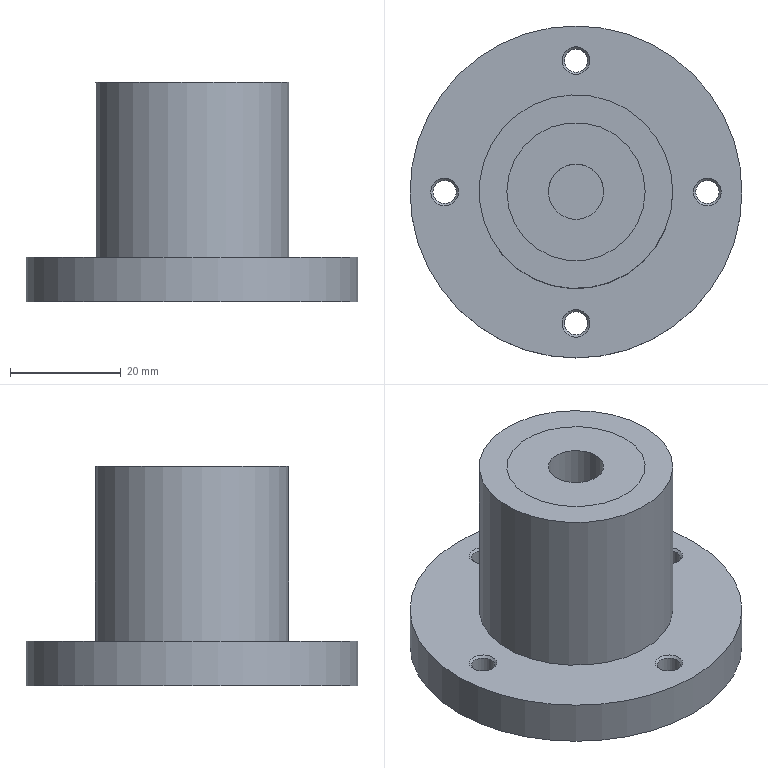Part | NX | features DATUM_CSYS 7, SKETCH 6, EXTRUDE 5, SIMPLE HOLE 4, SYMBOLIC_THREAD 4, HOLE PACKAGE 1 | 2 solids | 25 faces | box 60 x 60 x 39.6 mm | volume 47983 mm3 | cylinder 10 | cone 8 | plane 7 | commonest cylinder face diameters 4.2 x4 25 x2 10 x1 22 x1 35 x1 60 x1
STEP:
#1=CARTESIAN_POINT('',(30.,0.,8.));
#2=VERTEX_POINT('',#1);
#3=CARTESIAN_POINT('',(0.,0.,8.));
#4=DIRECTION('',(0.,0.,1.));
#5=DIRECTION('',(1.,0.,0.));
#6=AXIS2_PLACEMENT_3D('',#3,#4,#5);
#7=CIRCLE('',#6,30.);
#8=EDGE_CURVE('',#2,#2,#7,.T.);
#9=ORIENTED_EDGE('',*,*,#8,.F.);
#10=EDGE_LOOP('',(#9));
#11=FACE_BOUND('',#10,.T.);
#12=CARTESIAN_POINT('',(30.,0.,0.));
#13=VERTEX_POINT('',#12);
#14=CARTESIAN_POINT('',(0.,0.,0.));
#15=DIRECTION('',(0.,0.,1.));
#16=DIRECTION('',(1.,0.,0.));
#17=AXIS2_PLACEMENT_3D('',#14,#15,#16);
#18=CIRCLE('',#17,30.);
#19=EDGE_CURVE('',#13,#13,#18,.T.);
#20=ORIENTED_EDGE('',*,*,#19,.T.);
#21=EDGE_LOOP('',(#20));
#22=FACE_BOUND('',#21,.T.);
#23=CARTESIAN_POINT('',(0.,0.,8.));
#24=DIRECTION('',(0.,0.,-1.));
#25=DIRECTION('',(-1.,0.,0.));
#26=AXIS2_PLACEMENT_3D('',#23,#24,#25);
#27=CYLINDRICAL_SURFACE('',#26,30.);
#28=ADVANCED_FACE('',(#11,#22),#27,.T.);
#29=CARTESIAN_POINT('',(26.25,-0.00006047,8.));
#30=VERTEX_POINT('',#29);
#31=CARTESIAN_POINT('',(23.75,-0.00006047,8.));
#32=DIRECTION('',(0.,0.,1.));
#33=DIRECTION('',(1.,0.,0.));
#34=AXIS2_PLACEMENT_3D('',#31,#32,#33);
#35=CIRCLE('',#34,2.5);
#36=EDGE_CURVE('',#30,#30,#35,.F.);
#37=ORIENTED_EDGE('',*,*,#36,.T.);
#38=EDGE_LOOP('',(#37));
#39=FACE_BOUND('',#38,.T.);
#40=CARTESIAN_POINT('',(2.5,23.75,8.));
#41=VERTEX_POINT('',#40);
#42=CARTESIAN_POINT('',(0.00006047,23.75,8.));
#43=DIRECTION('',(0.,0.,1.));
#44=DIRECTION('',(1.,0.,0.));
#45=AXIS2_PLACEMENT_3D('',#42,#43,#44);
#46=CIRCLE('',#45,2.5);
#47=EDGE_CURVE('',#41,#41,#46,.F.);
#48=ORIENTED_EDGE('',*,*,#47,.T.);
#49=EDGE_LOOP('',(#48));
#50=FACE_BOUND('',#49,.T.);
#51=CARTESIAN_POINT('',(2.5,-23.75,8.));
#52=VERTEX_POINT('',#51);
#53=CARTESIAN_POINT('',(-0.00006047,-23.75,8.));
#54=DIRECTION('',(0.,0.,1.));
#55=DIRECTION('',(1.,0.,0.));
#56=AXIS2_PLACEMENT_3D('',#53,#54,#55);
#57=CIRCLE('',#56,2.5);
#58=EDGE_CURVE('',#52,#52,#57,.F.);
#59=ORIENTED_EDGE('',*,*,#58,.T.);
#60=EDGE_LOOP('',(#59));
#61=FACE_BOUND('',#60,.T.);
#62=CARTESIAN_POINT('',(-21.25,0.00006047,8.));
#63=VERTEX_POINT('',#62);
#64=CARTESIAN_POINT('',(-23.75,0.00006047,8.));
#65=DIRECTION('',(0.,0.,1.));
#66=DIRECTION('',(1.,0.,0.));
#67=AXIS2_PLACEMENT_3D('',#64,#65,#66);
#68=CIRCLE('',#67,2.5);
#69=EDGE_CURVE('',#63,#63,#68,.F.);
#70=ORIENTED_EDGE('',*,*,#69,.T.);
#71=EDGE_LOOP('',(#70));
#72=FACE_BOUND('',#71,.T.);
#73=CARTESIAN_POINT('',(17.5,0.,8.));
#74=VERTEX_POINT('',#73);
#75=CARTESIAN_POINT('',(0.,0.,8.));
#76=DIRECTION('',(0.,0.,1.));
#77=DIRECTION('',(1.,0.,0.));
#78=AXIS2_PLACEMENT_3D('',#75,#76,#77);
#79=CIRCLE('',#78,17.5);
#80=EDGE_CURVE('',#74,#74,#79,.T.);
#81=ORIENTED_EDGE('',*,*,#80,.F.);
#82=EDGE_LOOP('',(#81));
#83=FACE_BOUND('',#82,.T.);
#84=ORIENTED_EDGE('',*,*,#8,.T.);
#85=EDGE_LOOP('',(#84));
#86=FACE_BOUND('',#85,.T.);
#87=CARTESIAN_POINT('',(0.,0.,8.));
#88=DIRECTION('',(0.,0.,1.));
#89=DIRECTION('',(1.,0.,0.));
#90=AXIS2_PLACEMENT_3D('',#87,#88,#89);
#91=PLANE('',#90);
#92=ADVANCED_FACE('',(#39,#50,#61,#72,#83,#86),#91,.T.);
#93=CARTESIAN_POINT('',(26.25,-0.00006047,0.));
#94=VERTEX_POINT('',#93);
#95=CARTESIAN_POINT('',(23.75,-0.00006047,0.));
#96=DIRECTION('',(0.,0.,1.));
#97=DIRECTION('',(1.,0.,0.));
#98=AXIS2_PLACEMENT_3D('',#95,#96,#97);
#99=CIRCLE('',#98,2.5);
#100=EDGE_CURVE('',#94,#94,#99,.T.);
#101=ORIENTED_EDGE('',*,*,#100,.T.);
#102=EDGE_LOOP('',(#101));
#103=FACE_BOUND('',#102,.T.);
#104=CARTESIAN_POINT('',(2.5,23.75,0.));
#105=VERTEX_POINT('',#104);
#106=CARTESIAN_POINT('',(0.00006047,23.75,0.));
#107=DIRECTION('',(0.,0.,1.));
#108=DIRECTION('',(1.,0.,0.));
#109=AXIS2_PLACEMENT_3D('',#106,#107,#108);
#110=CIRCLE('',#109,2.5);
#111=EDGE_CURVE('',#105,#105,#110,.T.);
#112=ORIENTED_EDGE('',*,*,#111,.T.);
#113=EDGE_LOOP('',(#112));
#114=FACE_BOUND('',#113,.T.);
#115=CARTESIAN_POINT('',(2.5,-23.75,0.));
#116=VERTEX_POINT('',#115);
#117=CARTESIAN_POINT('',(-0.00006047,-23.75,0.));
#118=DIRECTION('',(0.,0.,1.));
#119=DIRECTION('',(1.,0.,0.));
#120=AXIS2_PLACEMENT_3D('',#117,#118,#119);
#121=CIRCLE('',#120,2.5);
#122=EDGE_CURVE('',#116,#116,#121,.T.);
#123=ORIENTED_EDGE('',*,*,#122,.T.);
#124=EDGE_LOOP('',(#123));
#125=FACE_BOUND('',#124,.T.);
#126=CARTESIAN_POINT('',(-21.25,0.00006047,0.));
#127=VERTEX_POINT('',#126);
#128=CARTESIAN_POINT('',(-23.75,0.00006047,0.));
#129=DIRECTION('',(0.,0.,1.));
#130=DIRECTION('',(1.,0.,0.));
#131=AXIS2_PLACEMENT_3D('',#128,#129,#130);
#132=CIRCLE('',#131,2.5);
#133=EDGE_CURVE('',#127,#127,#132,.T.);
#134=ORIENTED_EDGE('',*,*,#133,.T.);
#135=EDGE_LOOP('',(#134));
#136=FACE_BOUND('',#135,.T.);
#137=ORIENTED_EDGE('',*,*,#19,.F.);
#138=EDGE_LOOP('',(#137));
#139=FACE_BOUND('',#138,.T.);
#140=CARTESIAN_POINT('',(0.,0.,0.));
#141=DIRECTION('',(0.,0.,1.));
#142=DIRECTION('',(1.,0.,0.));
#143=AXIS2_PLACEMENT_3D('',#140,#141,#142);
#144=PLANE('',#143);
#145=ADVANCED_FACE('',(#103,#114,#125,#136,#139),#144,.F.);
#146=CARTESIAN_POINT('',(17.5,0.,39.6));
#147=VERTEX_POINT('',#146);
#148=CARTESIAN_POINT('',(0.,0.,39.6));
#149=DIRECTION('',(0.,0.,1.));
#150=DIRECTION('',(1.,0.,0.));
#151=AXIS2_PLACEMENT_3D('',#148,#149,#150);
#152=CIRCLE('',#151,17.5);
#153=EDGE_CURVE('',#147,#147,#152,.T.);
#154=ORIENTED_EDGE('',*,*,#153,.F.);
#155=EDGE_LOOP('',(#154));
#156=FACE_BOUND('',#155,.T.);
#157=ORIENTED_EDGE('',*,*,#80,.T.);
#158=EDGE_LOOP('',(#157));
#159=FACE_BOUND('',#158,.T.);
#160=CARTESIAN_POINT('',(0.,0.,39.6));
#161=DIRECTION('',(0.,0.,-1.));
#162=DIRECTION('',(-1.,0.,0.));
#163=AXIS2_PLACEMENT_3D('',#160,#161,#162);
#164=CYLINDRICAL_SURFACE('',#163,17.5);
#165=ADVANCED_FACE('',(#156,#159),#164,.T.);
#166=CARTESIAN_POINT('',(12.5,0.,39.6));
#167=VERTEX_POINT('',#166);
#168=CARTESIAN_POINT('',(0.,0.,39.6));
#169=DIRECTION('',(0.,0.,1.));
#170=DIRECTION('',(1.,0.,0.));
#171=AXIS2_PLACEMENT_3D('',#168,#169,#170);
#172=CIRCLE('',#171,12.5);
#173=EDGE_CURVE('',#167,#167,#172,.T.);
#174=ORIENTED_EDGE('',*,*,#173,.F.);
#175=EDGE_LOOP('',(#174));
#176=FACE_BOUND('',#175,.T.);
#177=ORIENTED_EDGE('',*,*,#153,.T.);
#178=EDGE_LOOP('',(#177));
#179=FACE_BOUND('',#178,.T.);
#180=CARTESIAN_POINT('',(0.,0.,39.6));
#181=DIRECTION('',(0.,0.,1.));
#182=DIRECTION('',(1.,0.,0.));
#183=AXIS2_PLACEMENT_3D('',#180,#181,#182);
#184=PLANE('',#183);
#185=ADVANCED_FACE('',(#176,#179),#184,.T.);
#186=CARTESIAN_POINT('',(12.5,0.,29.6));
#187=VERTEX_POINT('',#186);
#188=CARTESIAN_POINT('',(0.,0.,29.6));
#189=DIRECTION('',(0.,0.,1.));
#190=DIRECTION('',(1.,0.,0.));
#191=AXIS2_PLACEMENT_3D('',#188,#189,#190);
#192=CIRCLE('',#191,12.5);
#193=EDGE_CURVE('',#187,#187,#192,.F.);
#194=ORIENTED_EDGE('',*,*,#193,.T.);
#195=EDGE_LOOP('',(#194));
#196=FACE_BOUND('',#195,.T.);
#197=ORIENTED_EDGE('',*,*,#173,.T.);
#198=EDGE_LOOP('',(#197));
#199=FACE_BOUND('',#198,.T.);
#200=CARTESIAN_POINT('',(0.,0.,29.6));
#201=DIRECTION('',(0.,0.,1.));
#202=DIRECTION('',(1.,0.,0.));
#203=AXIS2_PLACEMENT_3D('',#200,#201,#202);
#204=CYLINDRICAL_SURFACE('',#203,12.5);
#205=ADVANCED_FACE('',(#196,#199),#204,.F.);
#206=CARTESIAN_POINT('',(11.,0.,29.6));
#207=VERTEX_POINT('',#206);
#208=CARTESIAN_POINT('',(0.,0.,29.6));
#209=DIRECTION('',(0.,0.,1.));
#210=DIRECTION('',(1.,0.,0.));
#211=AXIS2_PLACEMENT_3D('',#208,#209,#210);
#212=CIRCLE('',#211,11.);
#213=EDGE_CURVE('',#207,#207,#212,.T.);
#214=ORIENTED_EDGE('',*,*,#213,.F.);
#215=EDGE_LOOP('',(#214));
#216=FACE_BOUND('',#215,.T.);
#217=ORIENTED_EDGE('',*,*,#193,.F.);
#218=EDGE_LOOP('',(#217));
#219=FACE_BOUND('',#218,.T.);
#220=CARTESIAN_POINT('',(0.,0.,29.6));
#221=DIRECTION('',(0.,0.,1.));
#222=DIRECTION('',(1.,0.,0.));
#223=AXIS2_PLACEMENT_3D('',#220,#221,#222);
#224=PLANE('',#223);
#225=ADVANCED_FACE('',(#216,#219),#224,.T.);
#226=CARTESIAN_POINT('',(11.,0.,19.6));
#227=VERTEX_POINT('',#226);
#228=CARTESIAN_POINT('',(0.,0.,19.6));
#229=DIRECTION('',(0.,0.,1.));
#230=DIRECTION('',(1.,0.,0.));
#231=AXIS2_PLACEMENT_3D('',#228,#229,#230);
#232=CIRCLE('',#231,11.);
#233=EDGE_CURVE('',#227,#227,#232,.F.);
#234=ORIENTED_EDGE('',*,*,#233,.T.);
#235=EDGE_LOOP('',(#234));
#236=FACE_BOUND('',#235,.T.);
#237=ORIENTED_EDGE('',*,*,#213,.T.);
#238=EDGE_LOOP('',(#237));
#239=FACE_BOUND('',#238,.T.);
#240=CARTESIAN_POINT('',(0.,0.,19.6));
#241=DIRECTION('',(0.,0.,1.));
#242=DIRECTION('',(1.,0.,0.));
#243=AXIS2_PLACEMENT_3D('',#240,#241,#242);
#244=CYLINDRICAL_SURFACE('',#243,11.);
#245=ADVANCED_FACE('',(#236,#239),#244,.F.);
#246=ORIENTED_EDGE('',*,*,#233,.F.);
#247=EDGE_LOOP('',(#246));
#248=FACE_BOUND('',#247,.T.);
#249=CARTESIAN_POINT('',(0.,0.,19.6));
#250=DIRECTION('',(0.,0.,1.));
#251=DIRECTION('',(1.,0.,0.));
#252=AXIS2_PLACEMENT_3D('',#249,#250,#251);
#253=PLANE('',#252);
#254=ADVANCED_FACE('',(#248),#253,.T.);
#255=CARTESIAN_POINT('',(-21.65,0.00006047,0.4));
#256=VERTEX_POINT('',#255);
#257=CARTESIAN_POINT('',(-23.75,0.00006047,0.4));
#258=DIRECTION('',(0.,0.,1.));
#259=DIRECTION('',(1.,0.,0.));
#260=AXIS2_PLACEMENT_3D('',#257,#258,#259);
#261=CIRCLE('',#260,2.1);
#262=EDGE_CURVE('',#256,#256,#261,.F.);
#263=ORIENTED_EDGE('',*,*,#262,.T.);
#264=EDGE_LOOP('',(#263));
#265=FACE_BOUND('',#264,.T.);
#266=CARTESIAN_POINT('',(-21.65,0.00006047,7.6));
#267=VERTEX_POINT('',#266);
#268=CARTESIAN_POINT('',(-23.75,0.00006047,7.6));
#269=DIRECTION('',(0.,0.,1.));
#270=DIRECTION('',(1.,0.,0.));
#271=AXIS2_PLACEMENT_3D('',#268,#269,#270);
#272=CIRCLE('',#271,2.1);
#273=EDGE_CURVE('',#267,#267,#272,.T.);
#274=ORIENTED_EDGE('',*,*,#273,.T.);
#275=EDGE_LOOP('',(#274));
#276=FACE_BOUND('',#275,.T.);
#277=CARTESIAN_POINT('',(-23.75,0.00006047,8.));
#278=DIRECTION('',(0.,0.,-1.));
#279=DIRECTION('',(-1.,0.,0.));
#280=AXIS2_PLACEMENT_3D('',#277,#278,#279);
#281=CYLINDRICAL_SURFACE('',#280,2.1);
#282=ADVANCED_FACE('',(#265,#276),#281,.F.);
#283=ORIENTED_EDGE('',*,*,#273,.F.);
#284=EDGE_LOOP('',(#283));
#285=FACE_BOUND('',#284,.T.);
#286=ORIENTED_EDGE('',*,*,#69,.F.);
#287=EDGE_LOOP('',(#286));
#288=FACE_BOUND('',#287,.T.);
#289=CARTESIAN_POINT('',(-23.75,0.00006047,8.));
#290=DIRECTION('',(0.,0.,1.));
#291=DIRECTION('',(1.,0.,0.));
#292=AXIS2_PLACEMENT_3D('',#289,#290,#291);
#293=CONICAL_SURFACE('',#292,2.5,0.7854);
#294=ADVANCED_FACE('',(#285,#288),#293,.F.);
#295=ORIENTED_EDGE('',*,*,#262,.F.);
#296=EDGE_LOOP('',(#295));
#297=FACE_BOUND('',#296,.T.);
#298=ORIENTED_EDGE('',*,*,#133,.F.);
#299=EDGE_LOOP('',(#298));
#300=FACE_BOUND('',#299,.T.);
#301=CARTESIAN_POINT('',(-23.75,0.00006047,0.));
#302=DIRECTION('',(0.,0.,-1.));
#303=DIRECTION('',(-1.,0.,0.));
#304=AXIS2_PLACEMENT_3D('',#301,#302,#303);
#305=CONICAL_SURFACE('',#304,2.5,0.7854);
#306=ADVANCED_FACE('',(#297,#300),#305,.F.);
#307=CARTESIAN_POINT('',(2.1,-23.75,0.4));
#308=VERTEX_POINT('',#307);
#309=CARTESIAN_POINT('',(-0.00006047,-23.75,0.4));
#310=DIRECTION('',(0.,0.,1.));
#311=DIRECTION('',(1.,0.,0.));
#312=AXIS2_PLACEMENT_3D('',#309,#310,#311);
#313=CIRCLE('',#312,2.1);
#314=EDGE_CURVE('',#308,#308,#313,.F.);
#315=ORIENTED_EDGE('',*,*,#314,.T.);
#316=EDGE_LOOP('',(#315));
#317=FACE_BOUND('',#316,.T.);
#318=CARTESIAN_POINT('',(2.1,-23.75,7.6));
#319=VERTEX_POINT('',#318);
#320=CARTESIAN_POINT('',(-0.00006047,-23.75,7.6));
#321=DIRECTION('',(0.,0.,1.));
#322=DIRECTION('',(1.,0.,0.));
#323=AXIS2_PLACEMENT_3D('',#320,#321,#322);
#324=CIRCLE('',#323,2.1);
#325=EDGE_CURVE('',#319,#319,#324,.T.);
#326=ORIENTED_EDGE('',*,*,#325,.T.);
#327=EDGE_LOOP('',(#326));
#328=FACE_BOUND('',#327,.T.);
#329=CARTESIAN_POINT('',(-0.00006047,-23.75,8.));
#330=DIRECTION('',(0.,0.,-1.));
#331=DIRECTION('',(-1.,0.,0.));
#332=AXIS2_PLACEMENT_3D('',#329,#330,#331);
#333=CYLINDRICAL_SURFACE('',#332,2.1);
#334=ADVANCED_FACE('',(#317,#328),#333,.F.);
#335=ORIENTED_EDGE('',*,*,#325,.F.);
#336=EDGE_LOOP('',(#335));
#337=FACE_BOUND('',#336,.T.);
#338=ORIENTED_EDGE('',*,*,#58,.F.);
#339=EDGE_LOOP('',(#338));
#340=FACE_BOUND('',#339,.T.);
#341=CARTESIAN_POINT('',(-0.00006047,-23.75,8.));
#342=DIRECTION('',(0.,0.,1.));
#343=DIRECTION('',(1.,0.,0.));
#344=AXIS2_PLACEMENT_3D('',#341,#342,#343);
#345=CONICAL_SURFACE('',#344,2.5,0.7854);
#346=ADVANCED_FACE('',(#337,#340),#345,.F.);
#347=ORIENTED_EDGE('',*,*,#314,.F.);
#348=EDGE_LOOP('',(#347));
#349=FACE_BOUND('',#348,.T.);
#350=ORIENTED_EDGE('',*,*,#122,.F.);
#351=EDGE_LOOP('',(#350));
#352=FACE_BOUND('',#351,.T.);
#353=CARTESIAN_POINT('',(-0.00006047,-23.75,0.));
#354=DIRECTION('',(0.,0.,-1.));
#355=DIRECTION('',(-1.,0.,0.));
#356=AXIS2_PLACEMENT_3D('',#353,#354,#355);
#357=CONICAL_SURFACE('',#356,2.5,0.7854);
#358=ADVANCED_FACE('',(#349,#352),#357,.F.);
#359=CARTESIAN_POINT('',(2.1,23.75,0.4));
#360=VERTEX_POINT('',#359);
#361=CARTESIAN_POINT('',(0.00006047,23.75,0.4));
#362=DIRECTION('',(0.,0.,1.));
#363=DIRECTION('',(1.,0.,0.));
#364=AXIS2_PLACEMENT_3D('',#361,#362,#363);
#365=CIRCLE('',#364,2.1);
#366=EDGE_CURVE('',#360,#360,#365,.F.);
#367=ORIENTED_EDGE('',*,*,#366,.T.);
#368=EDGE_LOOP('',(#367));
#369=FACE_BOUND('',#368,.T.);
#370=CARTESIAN_POINT('',(2.1,23.75,7.6));
#371=VERTEX_POINT('',#370);
#372=CARTESIAN_POINT('',(0.00006047,23.75,7.6));
#373=DIRECTION('',(0.,0.,1.));
#374=DIRECTION('',(1.,0.,0.));
#375=AXIS2_PLACEMENT_3D('',#372,#373,#374);
#376=CIRCLE('',#375,2.1);
#377=EDGE_CURVE('',#371,#371,#376,.T.);
#378=ORIENTED_EDGE('',*,*,#377,.T.);
#379=EDGE_LOOP('',(#378));
#380=FACE_BOUND('',#379,.T.);
#381=CARTESIAN_POINT('',(0.00006047,23.75,8.));
#382=DIRECTION('',(0.,0.,-1.));
#383=DIRECTION('',(-1.,0.,0.));
#384=AXIS2_PLACEMENT_3D('',#381,#382,#383);
#385=CYLINDRICAL_SURFACE('',#384,2.1);
#386=ADVANCED_FACE('',(#369,#380),#385,.F.);
#387=ORIENTED_EDGE('',*,*,#377,.F.);
#388=EDGE_LOOP('',(#387));
#389=FACE_BOUND('',#388,.T.);
#390=ORIENTED_EDGE('',*,*,#47,.F.);
#391=EDGE_LOOP('',(#390));
#392=FACE_BOUND('',#391,.T.);
#393=CARTESIAN_POINT('',(0.00006047,23.75,8.));
#394=DIRECTION('',(0.,0.,1.));
#395=DIRECTION('',(1.,0.,0.));
#396=AXIS2_PLACEMENT_3D('',#393,#394,#395);
#397=CONICAL_SURFACE('',#396,2.5,0.7854);
#398=ADVANCED_FACE('',(#389,#392),#397,.F.);
#399=ORIENTED_EDGE('',*,*,#366,.F.);
#400=EDGE_LOOP('',(#399));
#401=FACE_BOUND('',#400,.T.);
#402=ORIENTED_EDGE('',*,*,#111,.F.);
#403=EDGE_LOOP('',(#402));
#404=FACE_BOUND('',#403,.T.);
#405=CARTESIAN_POINT('',(0.00006047,23.75,0.));
#406=DIRECTION('',(0.,0.,-1.));
#407=DIRECTION('',(-1.,0.,0.));
#408=AXIS2_PLACEMENT_3D('',#405,#406,#407);
#409=CONICAL_SURFACE('',#408,2.5,0.7854);
#410=ADVANCED_FACE('',(#401,#404),#409,.F.);
#411=CARTESIAN_POINT('',(25.85,-0.00006047,0.4));
#412=VERTEX_POINT('',#411);
#413=CARTESIAN_POINT('',(23.75,-0.00006047,0.4));
#414=DIRECTION('',(0.,0.,1.));
#415=DIRECTION('',(1.,0.,0.));
#416=AXIS2_PLACEMENT_3D('',#413,#414,#415);
#417=CIRCLE('',#416,2.1);
#418=EDGE_CURVE('',#412,#412,#417,.F.);
#419=ORIENTED_EDGE('',*,*,#418,.T.);
#420=EDGE_LOOP('',(#419));
#421=FACE_BOUND('',#420,.T.);
#422=CARTESIAN_POINT('',(25.85,-0.00006047,7.6));
#423=VERTEX_POINT('',#422);
#424=CARTESIAN_POINT('',(23.75,-0.00006047,7.6));
#425=DIRECTION('',(0.,0.,1.));
#426=DIRECTION('',(1.,0.,0.));
#427=AXIS2_PLACEMENT_3D('',#424,#425,#426);
#428=CIRCLE('',#427,2.1);
#429=EDGE_CURVE('',#423,#423,#428,.T.);
#430=ORIENTED_EDGE('',*,*,#429,.T.);
#431=EDGE_LOOP('',(#430));
#432=FACE_BOUND('',#431,.T.);
#433=CARTESIAN_POINT('',(23.75,-0.00006047,8.));
#434=DIRECTION('',(0.,0.,-1.));
#435=DIRECTION('',(-1.,0.,0.));
#436=AXIS2_PLACEMENT_3D('',#433,#434,#435);
#437=CYLINDRICAL_SURFACE('',#436,2.1);
#438=ADVANCED_FACE('',(#421,#432),#437,.F.);
#439=ORIENTED_EDGE('',*,*,#429,.F.);
#440=EDGE_LOOP('',(#439));
#441=FACE_BOUND('',#440,.T.);
#442=ORIENTED_EDGE('',*,*,#36,.F.);
#443=EDGE_LOOP('',(#442));
#444=FACE_BOUND('',#443,.T.);
#445=CARTESIAN_POINT('',(23.75,-0.00006047,8.));
#446=DIRECTION('',(0.,0.,1.));
#447=DIRECTION('',(1.,0.,0.));
#448=AXIS2_PLACEMENT_3D('',#445,#446,#447);
#449=CONICAL_SURFACE('',#448,2.5,0.7854);
#450=ADVANCED_FACE('',(#441,#444),#449,.F.);
#451=ORIENTED_EDGE('',*,*,#418,.F.);
#452=EDGE_LOOP('',(#451));
#453=FACE_BOUND('',#452,.T.);
#454=ORIENTED_EDGE('',*,*,#100,.F.);
#455=EDGE_LOOP('',(#454));
#456=FACE_BOUND('',#455,.T.);
#457=CARTESIAN_POINT('',(23.75,-0.00006047,0.));
#458=DIRECTION('',(0.,0.,-1.));
#459=DIRECTION('',(-1.,0.,0.));
#460=AXIS2_PLACEMENT_3D('',#457,#458,#459);
#461=CONICAL_SURFACE('',#460,2.5,0.7854);
#462=ADVANCED_FACE('',(#453,#456),#461,.F.);
#463=CLOSED_SHELL('',(#28,#92,#145,#165,#185,#205,#225,#245,#254,#282,#294,#306,#334,#346,#358,#386,#398,#410,#438,#450,#462));
#464=MANIFOLD_SOLID_BREP('',#463);
#465=CARTESIAN_POINT('',(12.5,0.,29.6));
#466=VERTEX_POINT('',#465);
#467=CARTESIAN_POINT('',(0.,0.,29.6));
#468=DIRECTION('',(0.,0.,1.));
#469=DIRECTION('',(1.,0.,0.));
#470=AXIS2_PLACEMENT_3D('',#467,#468,#469);
#471=CIRCLE('',#470,12.5);
#472=EDGE_CURVE('',#466,#466,#471,.T.);
#473=ORIENTED_EDGE('',*,*,#472,.T.);
#474=EDGE_LOOP('',(#473));
#475=FACE_BOUND('',#474,.T.);
#476=CARTESIAN_POINT('',(12.5,0.,39.6));
#477=VERTEX_POINT('',#476);
#478=CARTESIAN_POINT('',(0.,0.,39.6));
#479=DIRECTION('',(0.,0.,1.));
#480=DIRECTION('',(1.,0.,0.));
#481=AXIS2_PLACEMENT_3D('',#478,#479,#480);
#482=CIRCLE('',#481,12.5);
#483=EDGE_CURVE('',#477,#477,#482,.T.);
#484=ORIENTED_EDGE('',*,*,#483,.F.);
#485=EDGE_LOOP('',(#484));
#486=FACE_BOUND('',#485,.T.);
#487=CARTESIAN_POINT('',(0.,0.,29.6));
#488=DIRECTION('',(0.,0.,1.));
#489=DIRECTION('',(1.,0.,0.));
#490=AXIS2_PLACEMENT_3D('',#487,#488,#489);
#491=CYLINDRICAL_SURFACE('',#490,12.5);
#492=ADVANCED_FACE('',(#475,#486),#491,.T.);
#493=CARTESIAN_POINT('',(5.,0.,29.6));
#494=VERTEX_POINT('',#493);
#495=CARTESIAN_POINT('',(0.,0.,29.6));
#496=DIRECTION('',(0.,0.,1.));
#497=DIRECTION('',(1.,0.,0.));
#498=AXIS2_PLACEMENT_3D('',#495,#496,#497);
#499=CIRCLE('',#498,5.);
#500=EDGE_CURVE('',#494,#494,#499,.T.);
#501=ORIENTED_EDGE('',*,*,#500,.F.);
#502=EDGE_LOOP('',(#501));
#503=FACE_BOUND('',#502,.T.);
#504=CARTESIAN_POINT('',(5.,0.,39.6));
#505=VERTEX_POINT('',#504);
#506=CARTESIAN_POINT('',(0.,0.,39.6));
#507=DIRECTION('',(0.,0.,1.));
#508=DIRECTION('',(1.,0.,0.));
#509=AXIS2_PLACEMENT_3D('',#506,#507,#508);
#510=CIRCLE('',#509,5.);
#511=EDGE_CURVE('',#505,#505,#510,.T.);
#512=ORIENTED_EDGE('',*,*,#511,.T.);
#513=EDGE_LOOP('',(#512));
#514=FACE_BOUND('',#513,.T.);
#515=CARTESIAN_POINT('',(0.,0.,29.6));
#516=DIRECTION('',(0.,0.,1.));
#517=DIRECTION('',(1.,0.,0.));
#518=AXIS2_PLACEMENT_3D('',#515,#516,#517);
#519=CYLINDRICAL_SURFACE('',#518,5.);
#520=ADVANCED_FACE('',(#503,#514),#519,.F.);
#521=ORIENTED_EDGE('',*,*,#472,.F.);
#522=EDGE_LOOP('',(#521));
#523=FACE_BOUND('',#522,.T.);
#524=ORIENTED_EDGE('',*,*,#500,.T.);
#525=EDGE_LOOP('',(#524));
#526=FACE_BOUND('',#525,.T.);
#527=CARTESIAN_POINT('',(0.,0.,29.6));
#528=DIRECTION('',(0.,0.,1.));
#529=DIRECTION('',(1.,0.,0.));
#530=AXIS2_PLACEMENT_3D('',#527,#528,#529);
#531=PLANE('',#530);
#532=ADVANCED_FACE('',(#523,#526),#531,.F.);
#533=ORIENTED_EDGE('',*,*,#483,.T.);
#534=EDGE_LOOP('',(#533));
#535=FACE_BOUND('',#534,.T.);
#536=ORIENTED_EDGE('',*,*,#511,.F.);
#537=EDGE_LOOP('',(#536));
#538=FACE_BOUND('',#537,.T.);
#539=CARTESIAN_POINT('',(0.,0.,39.6));
#540=DIRECTION('',(0.,0.,1.));
#541=DIRECTION('',(1.,0.,0.));
#542=AXIS2_PLACEMENT_3D('',#539,#540,#541);
#543=PLANE('',#542);
#544=ADVANCED_FACE('',(#535,#538),#543,.T.);
#545=CLOSED_SHELL('',(#492,#520,#532,#544));
#546=MANIFOLD_SOLID_BREP('',#545);
#547=(LENGTH_UNIT()NAMED_UNIT(*)SI_UNIT(.MILLI.,.METRE.));
#548=UNCERTAINTY_MEASURE_WITH_UNIT(LENGTH_MEASURE(0.00001),#547,'','');
#549=(NAMED_UNIT(*)PLANE_ANGLE_UNIT()SI_UNIT($,.RADIAN.));
#550=(NAMED_UNIT(*)SI_UNIT($,.STERADIAN.)SOLID_ANGLE_UNIT());
#551=(GEOMETRIC_REPRESENTATION_CONTEXT(3)GLOBAL_UNCERTAINTY_ASSIGNED_CONTEXT((#548))GLOBAL_UNIT_ASSIGNED_CONTEXT((#547,#549,#550))REPRESENTATION_CONTEXT('',''));
#552=ADVANCED_BREP_SHAPE_REPRESENTATION('',(#464,#546),#551);